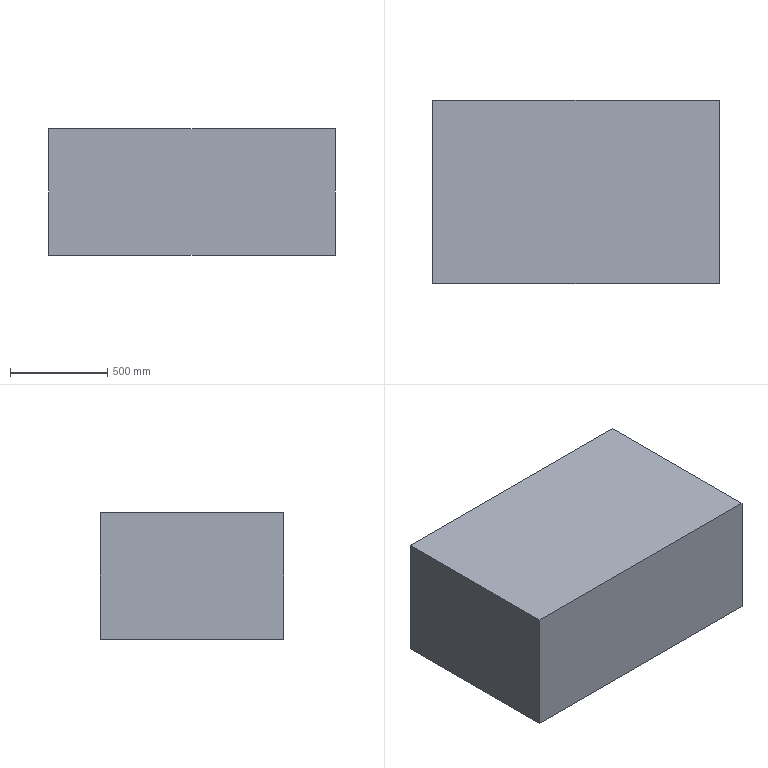Part | SolidWorks | features Extrusion 1, ICE 1 | 1 solid | 89 faces | box 1470 x 940 x 650 mm | volume 898157138 mm3 | plane 73 | spline 16